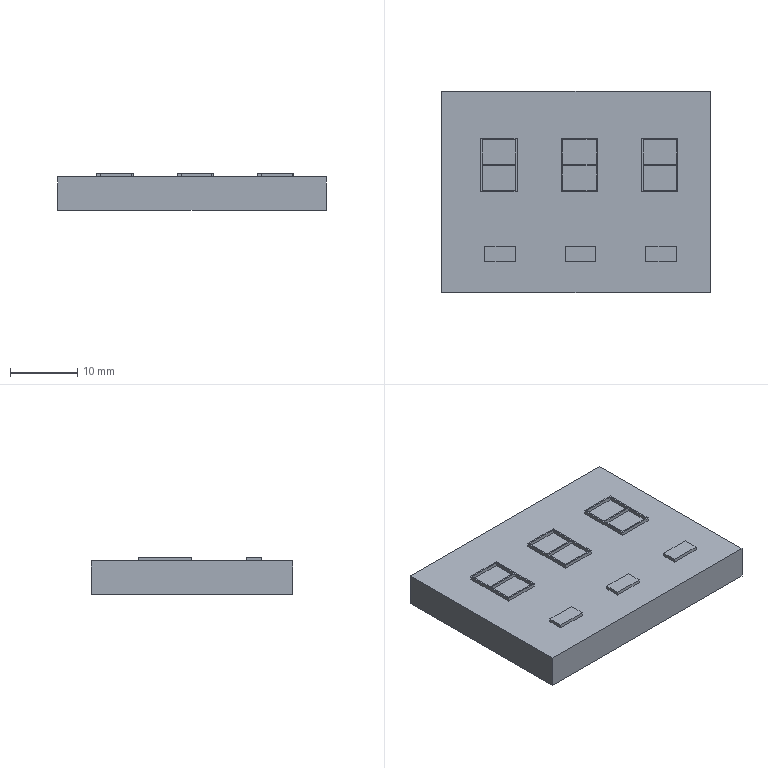Part | STEP file | DIP switch | 1 solid | 66 faces | box 40 x 30 x 5.5 mm | volume 6025 mm3 | plane 66